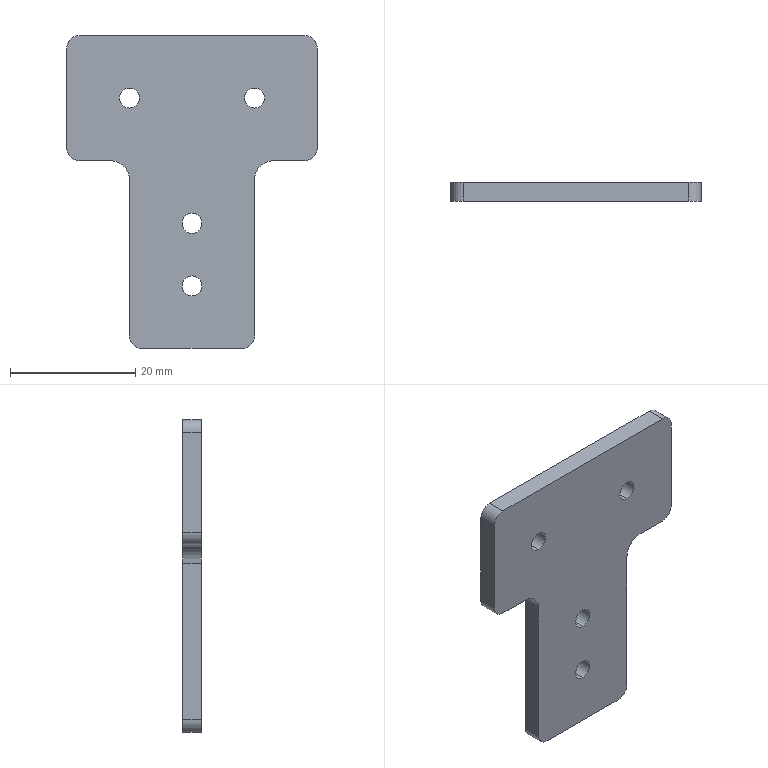Part | SolidWorks | features BaseBody 1 | 1 solid | 26 faces | box 40 x 3 x 50 mm | volume 4100 mm3 | cylinder 16 | plane 10 | commonest cylinder face diameters 3.2 x8 4 x6 6 x2
STEP:
#1=CARTESIAN_POINT('',(-10.,3.,16.6));
#2=VERTEX_POINT('',#1);
#3=CARTESIAN_POINT('',(-10.,3.,13.4));
#4=VERTEX_POINT('',#3);
#5=CARTESIAN_POINT('',(-10.,3.,15.));
#6=DIRECTION('',(0.,-1.,0.));
#7=DIRECTION('',(0.,0.,-1.));
#8=AXIS2_PLACEMENT_3D('',#5,#6,#7);
#9=CIRCLE('',#8,1.6);
#10=EDGE_CURVE('',#2,#4,#9,.T.);
#11=ORIENTED_EDGE('',*,*,#10,.F.);
#12=CARTESIAN_POINT('',(-10.,0.,16.6));
#13=VERTEX_POINT('',#12);
#14=CARTESIAN_POINT('',(-10.,3.,16.6));
#15=DIRECTION('',(0.,-1.,0.));
#16=VECTOR('',#15,1000.);
#17=LINE('',#14,#16);
#18=EDGE_CURVE('',#2,#13,#17,.T.);
#19=ORIENTED_EDGE('',*,*,#18,.T.);
#20=CARTESIAN_POINT('',(-10.,0.,13.4));
#21=VERTEX_POINT('',#20);
#22=CARTESIAN_POINT('',(-10.,0.,15.));
#23=DIRECTION('',(0.,-1.,0.));
#24=DIRECTION('',(0.,0.,-1.));
#25=AXIS2_PLACEMENT_3D('',#22,#23,#24);
#26=CIRCLE('',#25,1.6);
#27=EDGE_CURVE('',#13,#21,#26,.T.);
#28=ORIENTED_EDGE('',*,*,#27,.T.);
#29=CARTESIAN_POINT('',(-10.,3.,13.4));
#30=DIRECTION('',(0.,-1.,0.));
#31=VECTOR('',#30,1000.);
#32=LINE('',#29,#31);
#33=EDGE_CURVE('',#4,#21,#32,.T.);
#34=ORIENTED_EDGE('',*,*,#33,.F.);
#35=EDGE_LOOP('',(#11,#19,#28,#34));
#36=FACE_OUTER_BOUND('',#35,.T.);
#37=CARTESIAN_POINT('',(-10.,3.,15.));
#38=DIRECTION('',(0.,-1.,0.));
#39=DIRECTION('',(0.,0.,-1.));
#40=AXIS2_PLACEMENT_3D('',#37,#38,#39);
#41=CYLINDRICAL_SURFACE('',#40,1.6);
#42=ADVANCED_FACE('',(#36),#41,.F.);
#43=CARTESIAN_POINT('',(0.,3.,-13.4));
#44=VERTEX_POINT('',#43);
#45=CARTESIAN_POINT('',(0.,3.,-16.6));
#46=VERTEX_POINT('',#45);
#47=CARTESIAN_POINT('',(0.,3.,-15.));
#48=DIRECTION('',(0.,-1.,0.));
#49=DIRECTION('',(0.,0.,-1.));
#50=AXIS2_PLACEMENT_3D('',#47,#48,#49);
#51=CIRCLE('',#50,1.6);
#52=EDGE_CURVE('',#44,#46,#51,.T.);
#53=ORIENTED_EDGE('',*,*,#52,.F.);
#54=CARTESIAN_POINT('',(0.,0.,-13.4));
#55=VERTEX_POINT('',#54);
#56=CARTESIAN_POINT('',(0.,3.,-13.4));
#57=DIRECTION('',(0.,-1.,0.));
#58=VECTOR('',#57,1000.);
#59=LINE('',#56,#58);
#60=EDGE_CURVE('',#44,#55,#59,.T.);
#61=ORIENTED_EDGE('',*,*,#60,.T.);
#62=CARTESIAN_POINT('',(0.,0.,-16.6));
#63=VERTEX_POINT('',#62);
#64=CARTESIAN_POINT('',(0.,0.,-15.));
#65=DIRECTION('',(0.,-1.,0.));
#66=DIRECTION('',(0.,0.,-1.));
#67=AXIS2_PLACEMENT_3D('',#64,#65,#66);
#68=CIRCLE('',#67,1.6);
#69=EDGE_CURVE('',#55,#63,#68,.T.);
#70=ORIENTED_EDGE('',*,*,#69,.T.);
#71=CARTESIAN_POINT('',(0.,3.,-16.6));
#72=DIRECTION('',(0.,-1.,0.));
#73=VECTOR('',#72,1000.);
#74=LINE('',#71,#73);
#75=EDGE_CURVE('',#46,#63,#74,.T.);
#76=ORIENTED_EDGE('',*,*,#75,.F.);
#77=EDGE_LOOP('',(#53,#61,#70,#76));
#78=FACE_OUTER_BOUND('',#77,.T.);
#79=CARTESIAN_POINT('',(0.,3.,-15.));
#80=DIRECTION('',(0.,-1.,0.));
#81=DIRECTION('',(0.,0.,-1.));
#82=AXIS2_PLACEMENT_3D('',#79,#80,#81);
#83=CYLINDRICAL_SURFACE('',#82,1.6);
#84=ADVANCED_FACE('',(#78),#83,.F.);
#85=CARTESIAN_POINT('',(0.,3.,-3.4));
#86=VERTEX_POINT('',#85);
#87=CARTESIAN_POINT('',(0.,3.,-6.6));
#88=VERTEX_POINT('',#87);
#89=CARTESIAN_POINT('',(0.,3.,-5.));
#90=DIRECTION('',(0.,-1.,0.));
#91=DIRECTION('',(0.,0.,-1.));
#92=AXIS2_PLACEMENT_3D('',#89,#90,#91);
#93=CIRCLE('',#92,1.6);
#94=EDGE_CURVE('',#86,#88,#93,.T.);
#95=ORIENTED_EDGE('',*,*,#94,.F.);
#96=CARTESIAN_POINT('',(0.,0.,-3.4));
#97=VERTEX_POINT('',#96);
#98=CARTESIAN_POINT('',(0.,3.,-3.4));
#99=DIRECTION('',(0.,-1.,0.));
#100=VECTOR('',#99,1000.);
#101=LINE('',#98,#100);
#102=EDGE_CURVE('',#86,#97,#101,.T.);
#103=ORIENTED_EDGE('',*,*,#102,.T.);
#104=CARTESIAN_POINT('',(0.,0.,-6.6));
#105=VERTEX_POINT('',#104);
#106=CARTESIAN_POINT('',(0.,0.,-5.));
#107=DIRECTION('',(0.,-1.,0.));
#108=DIRECTION('',(0.,0.,-1.));
#109=AXIS2_PLACEMENT_3D('',#106,#107,#108);
#110=CIRCLE('',#109,1.6);
#111=EDGE_CURVE('',#97,#105,#110,.T.);
#112=ORIENTED_EDGE('',*,*,#111,.T.);
#113=CARTESIAN_POINT('',(0.,3.,-6.6));
#114=DIRECTION('',(0.,-1.,0.));
#115=VECTOR('',#114,1000.);
#116=LINE('',#113,#115);
#117=EDGE_CURVE('',#88,#105,#116,.T.);
#118=ORIENTED_EDGE('',*,*,#117,.F.);
#119=EDGE_LOOP('',(#95,#103,#112,#118));
#120=FACE_OUTER_BOUND('',#119,.T.);
#121=CARTESIAN_POINT('',(0.,3.,-5.));
#122=DIRECTION('',(0.,-1.,0.));
#123=DIRECTION('',(0.,0.,-1.));
#124=AXIS2_PLACEMENT_3D('',#121,#122,#123);
#125=CYLINDRICAL_SURFACE('',#124,1.6);
#126=ADVANCED_FACE('',(#120),#125,.F.);
#127=CARTESIAN_POINT('',(10.,3.,16.6));
#128=VERTEX_POINT('',#127);
#129=CARTESIAN_POINT('',(10.,3.,13.4));
#130=VERTEX_POINT('',#129);
#131=CARTESIAN_POINT('',(10.,3.,15.));
#132=DIRECTION('',(0.,-1.,0.));
#133=DIRECTION('',(0.,0.,-1.));
#134=AXIS2_PLACEMENT_3D('',#131,#132,#133);
#135=CIRCLE('',#134,1.6);
#136=EDGE_CURVE('',#128,#130,#135,.T.);
#137=ORIENTED_EDGE('',*,*,#136,.F.);
#138=CARTESIAN_POINT('',(10.,0.,16.6));
#139=VERTEX_POINT('',#138);
#140=CARTESIAN_POINT('',(10.,3.,16.6));
#141=DIRECTION('',(0.,-1.,0.));
#142=VECTOR('',#141,1000.);
#143=LINE('',#140,#142);
#144=EDGE_CURVE('',#128,#139,#143,.T.);
#145=ORIENTED_EDGE('',*,*,#144,.T.);
#146=CARTESIAN_POINT('',(10.,0.,13.4));
#147=VERTEX_POINT('',#146);
#148=CARTESIAN_POINT('',(10.,0.,15.));
#149=DIRECTION('',(0.,-1.,0.));
#150=DIRECTION('',(0.,0.,-1.));
#151=AXIS2_PLACEMENT_3D('',#148,#149,#150);
#152=CIRCLE('',#151,1.6);
#153=EDGE_CURVE('',#139,#147,#152,.T.);
#154=ORIENTED_EDGE('',*,*,#153,.T.);
#155=CARTESIAN_POINT('',(10.,3.,13.4));
#156=DIRECTION('',(0.,-1.,0.));
#157=VECTOR('',#156,1000.);
#158=LINE('',#155,#157);
#159=EDGE_CURVE('',#130,#147,#158,.T.);
#160=ORIENTED_EDGE('',*,*,#159,.F.);
#161=EDGE_LOOP('',(#137,#145,#154,#160));
#162=FACE_OUTER_BOUND('',#161,.T.);
#163=CARTESIAN_POINT('',(10.,3.,15.));
#164=DIRECTION('',(0.,-1.,0.));
#165=DIRECTION('',(0.,0.,-1.));
#166=AXIS2_PLACEMENT_3D('',#163,#164,#165);
#167=CYLINDRICAL_SURFACE('',#166,1.6);
#168=ADVANCED_FACE('',(#162),#167,.F.);
#169=CARTESIAN_POINT('',(-10.,0.,15.));
#170=DIRECTION('',(0.,-1.,0.));
#171=DIRECTION('',(0.,0.,-1.));
#172=AXIS2_PLACEMENT_3D('',#169,#170,#171);
#173=CIRCLE('',#172,1.6);
#174=EDGE_CURVE('',#21,#13,#173,.T.);
#175=ORIENTED_EDGE('',*,*,#174,.F.);
#176=ORIENTED_EDGE('',*,*,#27,.F.);
#177=EDGE_LOOP('',(#175,#176));
#178=FACE_BOUND('',#177,.T.);
#179=CARTESIAN_POINT('',(0.,0.,-15.));
#180=DIRECTION('',(0.,-1.,0.));
#181=DIRECTION('',(0.,0.,-1.));
#182=AXIS2_PLACEMENT_3D('',#179,#180,#181);
#183=CIRCLE('',#182,1.6);
#184=EDGE_CURVE('',#63,#55,#183,.T.);
#185=ORIENTED_EDGE('',*,*,#184,.F.);
#186=ORIENTED_EDGE('',*,*,#69,.F.);
#187=EDGE_LOOP('',(#185,#186));
#188=FACE_BOUND('',#187,.T.);
#189=CARTESIAN_POINT('',(0.,0.,-5.));
#190=DIRECTION('',(0.,-1.,0.));
#191=DIRECTION('',(0.,0.,-1.));
#192=AXIS2_PLACEMENT_3D('',#189,#190,#191);
#193=CIRCLE('',#192,1.6);
#194=EDGE_CURVE('',#105,#97,#193,.T.);
#195=ORIENTED_EDGE('',*,*,#194,.F.);
#196=ORIENTED_EDGE('',*,*,#111,.F.);
#197=EDGE_LOOP('',(#195,#196));
#198=FACE_BOUND('',#197,.T.);
#199=CARTESIAN_POINT('',(10.,0.,15.));
#200=DIRECTION('',(0.,-1.,0.));
#201=DIRECTION('',(0.,0.,-1.));
#202=AXIS2_PLACEMENT_3D('',#199,#200,#201);
#203=CIRCLE('',#202,1.6);
#204=EDGE_CURVE('',#147,#139,#203,.T.);
#205=ORIENTED_EDGE('',*,*,#204,.F.);
#206=ORIENTED_EDGE('',*,*,#153,.F.);
#207=EDGE_LOOP('',(#205,#206));
#208=FACE_BOUND('',#207,.T.);
#209=CARTESIAN_POINT('',(-18.,0.,5.));
#210=VERTEX_POINT('',#209);
#211=CARTESIAN_POINT('',(-20.,0.,7.));
#212=VERTEX_POINT('',#211);
#213=CARTESIAN_POINT('',(-18.,0.,7.));
#214=DIRECTION('',(0.,1.,0.));
#215=DIRECTION('',(0.,0.,1.));
#216=AXIS2_PLACEMENT_3D('',#213,#214,#215);
#217=CIRCLE('',#216,2.);
#218=EDGE_CURVE('',#210,#212,#217,.T.);
#219=ORIENTED_EDGE('',*,*,#218,.F.);
#220=CARTESIAN_POINT('',(-13.,0.,5.));
#221=VERTEX_POINT('',#220);
#222=CARTESIAN_POINT('',(0.,0.,5.));
#223=DIRECTION('',(-1.,0.,0.));
#224=VECTOR('',#223,1000.);
#225=LINE('',#222,#224);
#226=EDGE_CURVE('',#221,#210,#225,.T.);
#227=ORIENTED_EDGE('',*,*,#226,.F.);
#228=CARTESIAN_POINT('',(-10.,0.,2.));
#229=VERTEX_POINT('',#228);
#230=CARTESIAN_POINT('',(-13.,0.,2.));
#231=DIRECTION('',(0.,-1.,0.));
#232=DIRECTION('',(0.,0.,-1.));
#233=AXIS2_PLACEMENT_3D('',#230,#231,#232);
#234=CIRCLE('',#233,3.);
#235=EDGE_CURVE('',#229,#221,#234,.T.);
#236=ORIENTED_EDGE('',*,*,#235,.F.);
#237=CARTESIAN_POINT('',(-10.,0.,-23.));
#238=VERTEX_POINT('',#237);
#239=CARTESIAN_POINT('',(-10.,0.,0.));
#240=DIRECTION('',(0.,0.,1.));
#241=VECTOR('',#240,1000.);
#242=LINE('',#239,#241);
#243=EDGE_CURVE('',#238,#229,#242,.T.);
#244=ORIENTED_EDGE('',*,*,#243,.F.);
#245=CARTESIAN_POINT('',(-8.,0.,-25.));
#246=VERTEX_POINT('',#245);
#247=CARTESIAN_POINT('',(-8.,0.,-23.));
#248=DIRECTION('',(0.,1.,0.));
#249=DIRECTION('',(0.,0.,-1.));
#250=AXIS2_PLACEMENT_3D('',#247,#248,#249);
#251=CIRCLE('',#250,2.);
#252=EDGE_CURVE('',#246,#238,#251,.T.);
#253=ORIENTED_EDGE('',*,*,#252,.F.);
#254=CARTESIAN_POINT('',(8.,0.,-25.));
#255=VERTEX_POINT('',#254);
#256=CARTESIAN_POINT('',(0.,0.,-25.));
#257=DIRECTION('',(-1.,0.,0.));
#258=VECTOR('',#257,1000.);
#259=LINE('',#256,#258);
#260=EDGE_CURVE('',#255,#246,#259,.T.);
#261=ORIENTED_EDGE('',*,*,#260,.F.);
#262=CARTESIAN_POINT('',(10.,0.,-23.));
#263=VERTEX_POINT('',#262);
#264=CARTESIAN_POINT('',(8.,0.,-23.));
#265=DIRECTION('',(0.,1.,0.));
#266=DIRECTION('',(0.,0.,1.));
#267=AXIS2_PLACEMENT_3D('',#264,#265,#266);
#268=CIRCLE('',#267,2.);
#269=EDGE_CURVE('',#263,#255,#268,.T.);
#270=ORIENTED_EDGE('',*,*,#269,.F.);
#271=CARTESIAN_POINT('',(10.,0.,2.));
#272=VERTEX_POINT('',#271);
#273=CARTESIAN_POINT('',(10.,0.,0.));
#274=DIRECTION('',(0.,0.,-1.));
#275=VECTOR('',#274,1000.);
#276=LINE('',#273,#275);
#277=EDGE_CURVE('',#272,#263,#276,.T.);
#278=ORIENTED_EDGE('',*,*,#277,.F.);
#279=CARTESIAN_POINT('',(13.,0.,5.));
#280=VERTEX_POINT('',#279);
#281=CARTESIAN_POINT('',(13.,0.,2.));
#282=DIRECTION('',(0.,-1.,0.));
#283=DIRECTION('',(0.,0.,1.));
#284=AXIS2_PLACEMENT_3D('',#281,#282,#283);
#285=CIRCLE('',#284,3.);
#286=EDGE_CURVE('',#280,#272,#285,.T.);
#287=ORIENTED_EDGE('',*,*,#286,.F.);
#288=CARTESIAN_POINT('',(18.,0.,5.));
#289=VERTEX_POINT('',#288);
#290=CARTESIAN_POINT('',(0.,0.,5.));
#291=DIRECTION('',(-1.,0.,0.));
#292=VECTOR('',#291,1000.);
#293=LINE('',#290,#292);
#294=EDGE_CURVE('',#289,#280,#293,.T.);
#295=ORIENTED_EDGE('',*,*,#294,.F.);
#296=CARTESIAN_POINT('',(20.,0.,7.));
#297=VERTEX_POINT('',#296);
#298=CARTESIAN_POINT('',(18.,0.,7.));
#299=DIRECTION('',(0.,1.,0.));
#300=DIRECTION('',(0.,0.,-1.));
#301=AXIS2_PLACEMENT_3D('',#298,#299,#300);
#302=CIRCLE('',#301,2.);
#303=EDGE_CURVE('',#297,#289,#302,.T.);
#304=ORIENTED_EDGE('',*,*,#303,.F.);
#305=CARTESIAN_POINT('',(20.,0.,23.));
#306=VERTEX_POINT('',#305);
#307=CARTESIAN_POINT('',(20.,0.,0.));
#308=DIRECTION('',(0.,0.,-1.));
#309=VECTOR('',#308,1000.);
#310=LINE('',#307,#309);
#311=EDGE_CURVE('',#306,#297,#310,.T.);
#312=ORIENTED_EDGE('',*,*,#311,.F.);
#313=CARTESIAN_POINT('',(18.,0.,25.));
#314=VERTEX_POINT('',#313);
#315=CARTESIAN_POINT('',(18.,0.,23.));
#316=DIRECTION('',(0.,1.,0.));
#317=DIRECTION('',(0.,0.,-1.));
#318=AXIS2_PLACEMENT_3D('',#315,#316,#317);
#319=CIRCLE('',#318,2.);
#320=EDGE_CURVE('',#314,#306,#319,.T.);
#321=ORIENTED_EDGE('',*,*,#320,.F.);
#322=CARTESIAN_POINT('',(-18.,0.,25.));
#323=VERTEX_POINT('',#322);
#324=CARTESIAN_POINT('',(0.,0.,25.));
#325=DIRECTION('',(1.,0.,0.));
#326=VECTOR('',#325,1000.);
#327=LINE('',#324,#326);
#328=EDGE_CURVE('',#323,#314,#327,.T.);
#329=ORIENTED_EDGE('',*,*,#328,.F.);
#330=CARTESIAN_POINT('',(-20.,0.,23.));
#331=VERTEX_POINT('',#330);
#332=CARTESIAN_POINT('',(-18.,0.,23.));
#333=DIRECTION('',(0.,1.,0.));
#334=DIRECTION('',(0.,0.,1.));
#335=AXIS2_PLACEMENT_3D('',#332,#333,#334);
#336=CIRCLE('',#335,2.);
#337=EDGE_CURVE('',#331,#323,#336,.T.);
#338=ORIENTED_EDGE('',*,*,#337,.F.);
#339=CARTESIAN_POINT('',(-20.,0.,0.));
#340=DIRECTION('',(0.,0.,1.));
#341=VECTOR('',#340,1000.);
#342=LINE('',#339,#341);
#343=EDGE_CURVE('',#212,#331,#342,.T.);
#344=ORIENTED_EDGE('',*,*,#343,.F.);
#345=EDGE_LOOP('',(#219,#227,#236,#244,#253,#261,#270,#278,#287,#295,#304,#312,#321,#329,#338,#344));
#346=FACE_OUTER_BOUND('',#345,.T.);
#347=CARTESIAN_POINT('',(0.,0.,0.));
#348=DIRECTION('',(0.,1.,0.));
#349=DIRECTION('',(0.,0.,1.));
#350=AXIS2_PLACEMENT_3D('',#347,#348,#349);
#351=PLANE('',#350);
#352=ADVANCED_FACE('',(#178,#188,#198,#208,#346),#351,.F.);
#353=ORIENTED_EDGE('',*,*,#18,.F.);
#354=CARTESIAN_POINT('',(-10.,3.,15.));
#355=DIRECTION('',(0.,-1.,0.));
#356=DIRECTION('',(0.,0.,-1.));
#357=AXIS2_PLACEMENT_3D('',#354,#355,#356);
#358=CIRCLE('',#357,1.6);
#359=EDGE_CURVE('',#4,#2,#358,.T.);
#360=ORIENTED_EDGE('',*,*,#359,.F.);
#361=ORIENTED_EDGE('',*,*,#33,.T.);
#362=ORIENTED_EDGE('',*,*,#174,.T.);
#363=EDGE_LOOP('',(#353,#360,#361,#362));
#364=FACE_OUTER_BOUND('',#363,.T.);
#365=CARTESIAN_POINT('',(-10.,3.,15.));
#366=DIRECTION('',(0.,-1.,0.));
#367=DIRECTION('',(0.,0.,-1.));
#368=AXIS2_PLACEMENT_3D('',#365,#366,#367);
#369=CYLINDRICAL_SURFACE('',#368,1.6);
#370=ADVANCED_FACE('',(#364),#369,.F.);
#371=ORIENTED_EDGE('',*,*,#60,.F.);
#372=CARTESIAN_POINT('',(0.,3.,-15.));
#373=DIRECTION('',(0.,-1.,0.));
#374=DIRECTION('',(0.,0.,-1.));
#375=AXIS2_PLACEMENT_3D('',#372,#373,#374);
#376=CIRCLE('',#375,1.6);
#377=EDGE_CURVE('',#46,#44,#376,.T.);
#378=ORIENTED_EDGE('',*,*,#377,.F.);
#379=ORIENTED_EDGE('',*,*,#75,.T.);
#380=ORIENTED_EDGE('',*,*,#184,.T.);
#381=EDGE_LOOP('',(#371,#378,#379,#380));
#382=FACE_OUTER_BOUND('',#381,.T.);
#383=CARTESIAN_POINT('',(0.,3.,-15.));
#384=DIRECTION('',(0.,-1.,0.));
#385=DIRECTION('',(0.,0.,-1.));
#386=AXIS2_PLACEMENT_3D('',#383,#384,#385);
#387=CYLINDRICAL_SURFACE('',#386,1.6);
#388=ADVANCED_FACE('',(#382),#387,.F.);
#389=ORIENTED_EDGE('',*,*,#102,.F.);
#390=CARTESIAN_POINT('',(0.,3.,-5.));
#391=DIRECTION('',(0.,-1.,0.));
#392=DIRECTION('',(0.,0.,-1.));
#393=AXIS2_PLACEMENT_3D('',#390,#391,#392);
#394=CIRCLE('',#393,1.6);
#395=EDGE_CURVE('',#88,#86,#394,.T.);
#396=ORIENTED_EDGE('',*,*,#395,.F.);
#397=ORIENTED_EDGE('',*,*,#117,.T.);
#398=ORIENTED_EDGE('',*,*,#194,.T.);
#399=EDGE_LOOP('',(#389,#396,#397,#398));
#400=FACE_OUTER_BOUND('',#399,.T.);
#401=CARTESIAN_POINT('',(0.,3.,-5.));
#402=DIRECTION('',(0.,-1.,0.));
#403=DIRECTION('',(0.,0.,-1.));
#404=AXIS2_PLACEMENT_3D('',#401,#402,#403);
#405=CYLINDRICAL_SURFACE('',#404,1.6);
#406=ADVANCED_FACE('',(#400),#405,.F.);
#407=ORIENTED_EDGE('',*,*,#144,.F.);
#408=CARTESIAN_POINT('',(10.,3.,15.));
#409=DIRECTION('',(0.,-1.,0.));
#410=DIRECTION('',(0.,0.,-1.));
#411=AXIS2_PLACEMENT_3D('',#408,#409,#410);
#412=CIRCLE('',#411,1.6);
#413=EDGE_CURVE('',#130,#128,#412,.T.);
#414=ORIENTED_EDGE('',*,*,#413,.F.);
#415=ORIENTED_EDGE('',*,*,#159,.T.);
#416=ORIENTED_EDGE('',*,*,#204,.T.);
#417=EDGE_LOOP('',(#407,#414,#415,#416));
#418=FACE_OUTER_BOUND('',#417,.T.);
#419=CARTESIAN_POINT('',(10.,3.,15.));
#420=DIRECTION('',(0.,-1.,0.));
#421=DIRECTION('',(0.,0.,-1.));
#422=AXIS2_PLACEMENT_3D('',#419,#420,#421);
#423=CYLINDRICAL_SURFACE('',#422,1.6);
#424=ADVANCED_FACE('',(#418),#423,.F.);
#425=ORIENTED_EDGE('',*,*,#343,.T.);
#426=CARTESIAN_POINT('',(-20.,3.,23.));
#427=VERTEX_POINT('',#426);
#428=CARTESIAN_POINT('',(-20.,3.,23.));
#429=DIRECTION('',(0.,1.,0.));
#430=VECTOR('',#429,1000.);
#431=LINE('',#428,#430);
#432=EDGE_CURVE('',#331,#427,#431,.T.);
#433=ORIENTED_EDGE('',*,*,#432,.T.);
#434=CARTESIAN_POINT('',(-20.,3.,7.));
#435=VERTEX_POINT('',#434);
#436=CARTESIAN_POINT('',(-20.,3.,0.));
#437=DIRECTION('',(0.,0.,-1.));
#438=VECTOR('',#437,1000.);
#439=LINE('',#436,#438);
#440=EDGE_CURVE('',#427,#435,#439,.T.);
#441=ORIENTED_EDGE('',*,*,#440,.T.);
#442=CARTESIAN_POINT('',(-20.,3.,7.));
#443=DIRECTION('',(0.,-1.,0.));
#444=VECTOR('',#443,1000.);
#445=LINE('',#442,#444);
#446=EDGE_CURVE('',#435,#212,#445,.T.);
#447=ORIENTED_EDGE('',*,*,#446,.T.);
#448=EDGE_LOOP('',(#425,#433,#441,#447));
#449=FACE_OUTER_BOUND('',#448,.T.);
#450=CARTESIAN_POINT('',(-20.,3.,0.));
#451=DIRECTION('',(-1.,0.,0.));
#452=DIRECTION('',(0.,0.,1.));
#453=AXIS2_PLACEMENT_3D('',#450,#451,#452);
#454=PLANE('',#453);
#455=ADVANCED_FACE('',(#449),#454,.T.);
#456=ORIENTED_EDGE('',*,*,#218,.T.);
#457=ORIENTED_EDGE('',*,*,#446,.F.);
#458=CARTESIAN_POINT('',(-18.,3.,5.));
#459=VERTEX_POINT('',#458);
#460=CARTESIAN_POINT('',(-18.,3.,7.));
#461=DIRECTION('',(0.,-1.,0.));
#462=DIRECTION('',(0.,0.,1.));
#463=AXIS2_PLACEMENT_3D('',#460,#461,#462);
#464=CIRCLE('',#463,2.);
#465=EDGE_CURVE('',#435,#459,#464,.T.);
#466=ORIENTED_EDGE('',*,*,#465,.T.);
#467=CARTESIAN_POINT('',(-18.,3.,5.));
#468=DIRECTION('',(0.,-1.,0.));
#469=VECTOR('',#468,1000.);
#470=LINE('',#467,#469);
#471=EDGE_CURVE('',#459,#210,#470,.T.);
#472=ORIENTED_EDGE('',*,*,#471,.T.);
#473=EDGE_LOOP('',(#456,#457,#466,#472));
#474=FACE_OUTER_BOUND('',#473,.T.);
#475=CARTESIAN_POINT('',(-18.,3.,7.));
#476=DIRECTION('',(0.,1.,0.));
#477=DIRECTION('',(0.,0.,1.));
#478=AXIS2_PLACEMENT_3D('',#475,#476,#477);
#479=CYLINDRICAL_SURFACE('',#478,2.);
#480=ADVANCED_FACE('',(#474),#479,.T.);
#481=ORIENTED_EDGE('',*,*,#471,.F.);
#482=CARTESIAN_POINT('',(-13.,3.,5.));
#483=VERTEX_POINT('',#482);
#484=CARTESIAN_POINT('',(0.,3.,5.));
#485=DIRECTION('',(-1.,0.,0.));
#486=VECTOR('',#485,1000.);
#487=LINE('',#484,#486);
#488=EDGE_CURVE('',#483,#459,#487,.T.);
#489=ORIENTED_EDGE('',*,*,#488,.F.);
#490=CARTESIAN_POINT('',(-13.,3.,5.));
#491=DIRECTION('',(0.,1.,0.));
#492=VECTOR('',#491,1000.);
#493=LINE('',#490,#492);
#494=EDGE_CURVE('',#221,#483,#493,.T.);
#495=ORIENTED_EDGE('',*,*,#494,.F.);
#496=ORIENTED_EDGE('',*,*,#226,.T.);
#497=EDGE_LOOP('',(#481,#489,#495,#496));
#498=FACE_OUTER_BOUND('',#497,.T.);
#499=CARTESIAN_POINT('',(0.,3.,5.));
#500=DIRECTION('',(0.,0.,1.));
#501=DIRECTION('',(1.,0.,0.));
#502=AXIS2_PLACEMENT_3D('',#499,#500,#501);
#503=PLANE('',#502);
#504=ADVANCED_FACE('',(#498),#503,.F.);
#505=CARTESIAN_POINT('',(-10.,3.,2.));
#506=VERTEX_POINT('',#505);
#507=CARTESIAN_POINT('',(-10.,3.,2.));
#508=DIRECTION('',(0.,1.,0.));
#509=VECTOR('',#508,1000.);
#510=LINE('',#507,#509);
#511=EDGE_CURVE('',#229,#506,#510,.T.);
#512=ORIENTED_EDGE('',*,*,#511,.F.);
#513=ORIENTED_EDGE('',*,*,#235,.T.);
#514=ORIENTED_EDGE('',*,*,#494,.T.);
#515=CARTESIAN_POINT('',(-13.,3.,2.));
#516=DIRECTION('',(0.,-1.,0.));
#517=DIRECTION('',(0.,0.,-1.));
#518=AXIS2_PLACEMENT_3D('',#515,#516,#517);
#519=CIRCLE('',#518,3.);
#520=EDGE_CURVE('',#506,#483,#519,.T.);
#521=ORIENTED_EDGE('',*,*,#520,.F.);
#522=EDGE_LOOP('',(#512,#513,#514,#521));
#523=FACE_OUTER_BOUND('',#522,.T.);
#524=CARTESIAN_POINT('',(-13.,3.,2.));
#525=DIRECTION('',(0.,-1.,0.));
#526=DIRECTION('',(0.,0.,-1.));
#527=AXIS2_PLACEMENT_3D('',#524,#525,#526);
#528=CYLINDRICAL_SURFACE('',#527,3.);
#529=ADVANCED_FACE('',(#523),#528,.F.);
#530=ORIENTED_EDGE('',*,*,#243,.T.);
#531=ORIENTED_EDGE('',*,*,#511,.T.);
#532=CARTESIAN_POINT('',(-10.,3.,-23.));
#533=VERTEX_POINT('',#532);
#534=CARTESIAN_POINT('',(-10.,3.,0.));
#535=DIRECTION('',(0.,0.,-1.));
#536=VECTOR('',#535,1000.);
#537=LINE('',#534,#536);
#538=EDGE_CURVE('',#506,#533,#537,.T.);
#539=ORIENTED_EDGE('',*,*,#538,.T.);
#540=CARTESIAN_POINT('',(-10.,3.,-23.));
#541=DIRECTION('',(0.,-1.,0.));
#542=VECTOR('',#541,1000.);
#543=LINE('',#540,#542);
#544=EDGE_CURVE('',#533,#238,#543,.T.);
#545=ORIENTED_EDGE('',*,*,#544,.T.);
#546=EDGE_LOOP('',(#530,#531,#539,#545));
#547=FACE_OUTER_BOUND('',#546,.T.);
#548=CARTESIAN_POINT('',(-10.,3.,0.));
#549=DIRECTION('',(-1.,0.,0.));
#550=DIRECTION('',(0.,0.,1.));
#551=AXIS2_PLACEMENT_3D('',#548,#549,#550);
#552=PLANE('',#551);
#553=ADVANCED_FACE('',(#547),#552,.T.);
#554=ORIENTED_EDGE('',*,*,#252,.T.);
#555=ORIENTED_EDGE('',*,*,#544,.F.);
#556=CARTESIAN_POINT('',(-8.,3.,-25.));
#557=VERTEX_POINT('',#556);
#558=CARTESIAN_POINT('',(-8.,3.,-23.));
#559=DIRECTION('',(0.,-1.,0.));
#560=DIRECTION('',(0.,0.,-1.));
#561=AXIS2_PLACEMENT_3D('',#558,#559,#560);
#562=CIRCLE('',#561,2.);
#563=EDGE_CURVE('',#533,#557,#562,.T.);
#564=ORIENTED_EDGE('',*,*,#563,.T.);
#565=CARTESIAN_POINT('',(-8.,3.,-25.));
#566=DIRECTION('',(0.,-1.,0.));
#567=VECTOR('',#566,1000.);
#568=LINE('',#565,#567);
#569=EDGE_CURVE('',#557,#246,#568,.T.);
#570=ORIENTED_EDGE('',*,*,#569,.T.);
#571=EDGE_LOOP('',(#554,#555,#564,#570));
#572=FACE_OUTER_BOUND('',#571,.T.);
#573=CARTESIAN_POINT('',(-8.,3.,-23.));
#574=DIRECTION('',(0.,-1.,0.));
#575=DIRECTION('',(0.,0.,-1.));
#576=AXIS2_PLACEMENT_3D('',#573,#574,#575);
#577=CYLINDRICAL_SURFACE('',#576,2.);
#578=ADVANCED_FACE('',(#572),#577,.T.);
#579=ORIENTED_EDGE('',*,*,#260,.T.);
#580=ORIENTED_EDGE('',*,*,#569,.F.);
#581=CARTESIAN_POINT('',(8.,3.,-25.));
#582=VERTEX_POINT('',#581);
#583=CARTESIAN_POINT('',(0.,3.,-25.));
#584=DIRECTION('',(1.,0.,0.));
#585=VECTOR('',#584,1000.);
#586=LINE('',#583,#585);
#587=EDGE_CURVE('',#557,#582,#586,.T.);
#588=ORIENTED_EDGE('',*,*,#587,.T.);
#589=CARTESIAN_POINT('',(8.,3.,-25.));
#590=DIRECTION('',(0.,-1.,0.));
#591=VECTOR('',#590,1000.);
#592=LINE('',#589,#591);
#593=EDGE_CURVE('',#582,#255,#592,.T.);
#594=ORIENTED_EDGE('',*,*,#593,.T.);
#595=EDGE_LOOP('',(#579,#580,#588,#594));
#596=FACE_OUTER_BOUND('',#595,.T.);
#597=CARTESIAN_POINT('',(0.,3.,-25.));
#598=DIRECTION('',(0.,0.,-1.));
#599=DIRECTION('',(-1.,0.,0.));
#600=AXIS2_PLACEMENT_3D('',#597,#598,#599);
#601=PLANE('',#600);
#602=ADVANCED_FACE('',(#596),#601,.T.);
#603=ORIENTED_EDGE('',*,*,#269,.T.);
#604=ORIENTED_EDGE('',*,*,#593,.F.);
#605=CARTESIAN_POINT('',(10.,3.,-23.));
#606=VERTEX_POINT('',#605);
#607=CARTESIAN_POINT('',(8.,3.,-23.));
#608=DIRECTION('',(0.,-1.,0.));
#609=DIRECTION('',(0.,0.,1.));
#610=AXIS2_PLACEMENT_3D('',#607,#608,#609);
#611=CIRCLE('',#610,2.);
#612=EDGE_CURVE('',#582,#606,#611,.T.);
#613=ORIENTED_EDGE('',*,*,#612,.T.);
#614=CARTESIAN_POINT('',(10.,3.,-23.));
#615=DIRECTION('',(0.,-1.,0.));
#616=VECTOR('',#615,1000.);
#617=LINE('',#614,#616);
#618=EDGE_CURVE('',#606,#263,#617,.T.);
#619=ORIENTED_EDGE('',*,*,#618,.T.);
#620=EDGE_LOOP('',(#603,#604,#613,#619));
#621=FACE_OUTER_BOUND('',#620,.T.);
#622=CARTESIAN_POINT('',(8.,3.,-23.));
#623=DIRECTION('',(0.,1.,0.));
#624=DIRECTION('',(0.,0.,1.));
#625=AXIS2_PLACEMENT_3D('',#622,#623,#624);
#626=CYLINDRICAL_SURFACE('',#625,2.);
#627=ADVANCED_FACE('',(#621),#626,.T.);
#628=ORIENTED_EDGE('',*,*,#618,.F.);
#629=CARTESIAN_POINT('',(10.,3.,2.));
#630=VERTEX_POINT('',#629);
#631=CARTESIAN_POINT('',(10.,3.,0.));
#632=DIRECTION('',(0.,0.,-1.));
#633=VECTOR('',#632,1000.);
#634=LINE('',#631,#633);
#635=EDGE_CURVE('',#630,#606,#634,.T.);
#636=ORIENTED_EDGE('',*,*,#635,.F.);
#637=CARTESIAN_POINT('',(10.,3.,2.));
#638=DIRECTION('',(0.,1.,0.));
#639=VECTOR('',#638,1000.);
#640=LINE('',#637,#639);
#641=EDGE_CURVE('',#272,#630,#640,.T.);
#642=ORIENTED_EDGE('',*,*,#641,.F.);
#643=ORIENTED_EDGE('',*,*,#277,.T.);
#644=EDGE_LOOP('',(#628,#636,#642,#643));
#645=FACE_OUTER_BOUND('',#644,.T.);
#646=CARTESIAN_POINT('',(10.,3.,0.));
#647=DIRECTION('',(-1.,0.,0.));
#648=DIRECTION('',(0.,0.,1.));
#649=AXIS2_PLACEMENT_3D('',#646,#647,#648);
#650=PLANE('',#649);
#651=ADVANCED_FACE('',(#645),#650,.F.);
#652=CARTESIAN_POINT('',(13.,3.,5.));
#653=VERTEX_POINT('',#652);
#654=CARTESIAN_POINT('',(13.,3.,5.));
#655=DIRECTION('',(0.,1.,0.));
#656=VECTOR('',#655,1000.);
#657=LINE('',#654,#656);
#658=EDGE_CURVE('',#280,#653,#657,.T.);
#659=ORIENTED_EDGE('',*,*,#658,.F.);
#660=ORIENTED_EDGE('',*,*,#286,.T.);
#661=ORIENTED_EDGE('',*,*,#641,.T.);
#662=CARTESIAN_POINT('',(13.,3.,2.));
#663=DIRECTION('',(0.,-1.,0.));
#664=DIRECTION('',(0.,0.,1.));
#665=AXIS2_PLACEMENT_3D('',#662,#663,#664);
#666=CIRCLE('',#665,3.);
#667=EDGE_CURVE('',#653,#630,#666,.T.);
#668=ORIENTED_EDGE('',*,*,#667,.F.);
#669=EDGE_LOOP('',(#659,#660,#661,#668));
#670=FACE_OUTER_BOUND('',#669,.T.);
#671=CARTESIAN_POINT('',(13.,3.,2.));
#672=DIRECTION('',(0.,1.,0.));
#673=DIRECTION('',(0.,0.,1.));
#674=AXIS2_PLACEMENT_3D('',#671,#672,#673);
#675=CYLINDRICAL_SURFACE('',#674,3.);
#676=ADVANCED_FACE('',(#670),#675,.F.);
#677=CARTESIAN_POINT('',(18.,3.,5.));
#678=VERTEX_POINT('',#677);
#679=CARTESIAN_POINT('',(18.,3.,5.));
#680=DIRECTION('',(0.,1.,0.));
#681=VECTOR('',#680,1000.);
#682=LINE('',#679,#681);
#683=EDGE_CURVE('',#289,#678,#682,.T.);
#684=ORIENTED_EDGE('',*,*,#683,.F.);
#685=ORIENTED_EDGE('',*,*,#294,.T.);
#686=ORIENTED_EDGE('',*,*,#658,.T.);
#687=CARTESIAN_POINT('',(0.,3.,5.));
#688=DIRECTION('',(-1.,0.,0.));
#689=VECTOR('',#688,1000.);
#690=LINE('',#687,#689);
#691=EDGE_CURVE('',#678,#653,#690,.T.);
#692=ORIENTED_EDGE('',*,*,#691,.F.);
#693=EDGE_LOOP('',(#684,#685,#686,#692));
#694=FACE_OUTER_BOUND('',#693,.T.);
#695=CARTESIAN_POINT('',(0.,3.,5.));
#696=DIRECTION('',(0.,0.,1.));
#697=DIRECTION('',(1.,0.,0.));
#698=AXIS2_PLACEMENT_3D('',#695,#696,#697);
#699=PLANE('',#698);
#700=ADVANCED_FACE('',(#694),#699,.F.);
#701=ORIENTED_EDGE('',*,*,#303,.T.);
#702=ORIENTED_EDGE('',*,*,#683,.T.);
#703=CARTESIAN_POINT('',(20.,3.,7.));
#704=VERTEX_POINT('',#703);
#705=CARTESIAN_POINT('',(18.,3.,7.));
#706=DIRECTION('',(0.,-1.,0.));
#707=DIRECTION('',(0.,0.,-1.));
#708=AXIS2_PLACEMENT_3D('',#705,#706,#707);
#709=CIRCLE('',#708,2.);
#710=EDGE_CURVE('',#678,#704,#709,.T.);
#711=ORIENTED_EDGE('',*,*,#710,.T.);
#712=CARTESIAN_POINT('',(20.,3.,7.));
#713=DIRECTION('',(0.,-1.,0.));
#714=VECTOR('',#713,1000.);
#715=LINE('',#712,#714);
#716=EDGE_CURVE('',#704,#297,#715,.T.);
#717=ORIENTED_EDGE('',*,*,#716,.T.);
#718=EDGE_LOOP('',(#701,#702,#711,#717));
#719=FACE_OUTER_BOUND('',#718,.T.);
#720=CARTESIAN_POINT('',(18.,3.,7.));
#721=DIRECTION('',(0.,-1.,0.));
#722=DIRECTION('',(0.,0.,-1.));
#723=AXIS2_PLACEMENT_3D('',#720,#721,#722);
#724=CYLINDRICAL_SURFACE('',#723,2.);
#725=ADVANCED_FACE('',(#719),#724,.T.);
#726=CARTESIAN_POINT('',(20.,3.,23.));
#727=VERTEX_POINT('',#726);
#728=CARTESIAN_POINT('',(20.,3.,23.));
#729=DIRECTION('',(0.,1.,0.));
#730=VECTOR('',#729,1000.);
#731=LINE('',#728,#730);
#732=EDGE_CURVE('',#306,#727,#731,.T.);
#733=ORIENTED_EDGE('',*,*,#732,.F.);
#734=ORIENTED_EDGE('',*,*,#311,.T.);
#735=ORIENTED_EDGE('',*,*,#716,.F.);
#736=CARTESIAN_POINT('',(20.,3.,0.));
#737=DIRECTION('',(0.,0.,-1.));
#738=VECTOR('',#737,1000.);
#739=LINE('',#736,#738);
#740=EDGE_CURVE('',#727,#704,#739,.T.);
#741=ORIENTED_EDGE('',*,*,#740,.F.);
#742=EDGE_LOOP('',(#733,#734,#735,#741));
#743=FACE_OUTER_BOUND('',#742,.T.);
#744=CARTESIAN_POINT('',(20.,3.,0.));
#745=DIRECTION('',(-1.,0.,0.));
#746=DIRECTION('',(0.,0.,1.));
#747=AXIS2_PLACEMENT_3D('',#744,#745,#746);
#748=PLANE('',#747);
#749=ADVANCED_FACE('',(#743),#748,.F.);
#750=ORIENTED_EDGE('',*,*,#320,.T.);
#751=ORIENTED_EDGE('',*,*,#732,.T.);
#752=CARTESIAN_POINT('',(18.,3.,25.));
#753=VERTEX_POINT('',#752);
#754=CARTESIAN_POINT('',(18.,3.,23.));
#755=DIRECTION('',(0.,-1.,0.));
#756=DIRECTION('',(0.,0.,-1.));
#757=AXIS2_PLACEMENT_3D('',#754,#755,#756);
#758=CIRCLE('',#757,2.);
#759=EDGE_CURVE('',#727,#753,#758,.T.);
#760=ORIENTED_EDGE('',*,*,#759,.T.);
#761=CARTESIAN_POINT('',(18.,3.,25.));
#762=DIRECTION('',(0.,-1.,0.));
#763=VECTOR('',#762,1000.);
#764=LINE('',#761,#763);
#765=EDGE_CURVE('',#753,#314,#764,.T.);
#766=ORIENTED_EDGE('',*,*,#765,.T.);
#767=EDGE_LOOP('',(#750,#751,#760,#766));
#768=FACE_OUTER_BOUND('',#767,.T.);
#769=CARTESIAN_POINT('',(18.,3.,23.));
#770=DIRECTION('',(0.,-1.,0.));
#771=DIRECTION('',(0.,0.,-1.));
#772=AXIS2_PLACEMENT_3D('',#769,#770,#771);
#773=CYLINDRICAL_SURFACE('',#772,2.);
#774=ADVANCED_FACE('',(#768),#773,.T.);
#775=CARTESIAN_POINT('',(-18.,3.,25.));
#776=VERTEX_POINT('',#775);
#777=CARTESIAN_POINT('',(-18.,3.,25.));
#778=DIRECTION('',(0.,1.,0.));
#779=VECTOR('',#778,1000.);
#780=LINE('',#777,#779);
#781=EDGE_CURVE('',#323,#776,#780,.T.);
#782=ORIENTED_EDGE('',*,*,#781,.F.);
#783=ORIENTED_EDGE('',*,*,#328,.T.);
#784=ORIENTED_EDGE('',*,*,#765,.F.);
#785=CARTESIAN_POINT('',(0.,3.,25.));
#786=DIRECTION('',(1.,0.,0.));
#787=VECTOR('',#786,1000.);
#788=LINE('',#785,#787);
#789=EDGE_CURVE('',#776,#753,#788,.T.);
#790=ORIENTED_EDGE('',*,*,#789,.F.);
#791=EDGE_LOOP('',(#782,#783,#784,#790));
#792=FACE_OUTER_BOUND('',#791,.T.);
#793=CARTESIAN_POINT('',(0.,3.,25.));
#794=DIRECTION('',(0.,0.,-1.));
#795=DIRECTION('',(-1.,0.,0.));
#796=AXIS2_PLACEMENT_3D('',#793,#794,#795);
#797=PLANE('',#796);
#798=ADVANCED_FACE('',(#792),#797,.F.);
#799=ORIENTED_EDGE('',*,*,#337,.T.);
#800=ORIENTED_EDGE('',*,*,#781,.T.);
#801=CARTESIAN_POINT('',(-18.,3.,23.));
#802=DIRECTION('',(0.,-1.,0.));
#803=DIRECTION('',(0.,0.,1.));
#804=AXIS2_PLACEMENT_3D('',#801,#802,#803);
#805=CIRCLE('',#804,2.);
#806=EDGE_CURVE('',#776,#427,#805,.T.);
#807=ORIENTED_EDGE('',*,*,#806,.T.);
#808=ORIENTED_EDGE('',*,*,#432,.F.);
#809=EDGE_LOOP('',(#799,#800,#807,#808));
#810=FACE_OUTER_BOUND('',#809,.T.);
#811=CARTESIAN_POINT('',(-18.,3.,23.));
#812=DIRECTION('',(0.,1.,0.));
#813=DIRECTION('',(0.,0.,1.));
#814=AXIS2_PLACEMENT_3D('',#811,#812,#813);
#815=CYLINDRICAL_SURFACE('',#814,2.);
#816=ADVANCED_FACE('',(#810),#815,.T.);
#817=ORIENTED_EDGE('',*,*,#359,.T.);
#818=ORIENTED_EDGE('',*,*,#10,.T.);
#819=EDGE_LOOP('',(#817,#818));
#820=FACE_BOUND('',#819,.T.);
#821=ORIENTED_EDGE('',*,*,#377,.T.);
#822=ORIENTED_EDGE('',*,*,#52,.T.);
#823=EDGE_LOOP('',(#821,#822));
#824=FACE_BOUND('',#823,.T.);
#825=ORIENTED_EDGE('',*,*,#395,.T.);
#826=ORIENTED_EDGE('',*,*,#94,.T.);
#827=EDGE_LOOP('',(#825,#826));
#828=FACE_BOUND('',#827,.T.);
#829=ORIENTED_EDGE('',*,*,#413,.T.);
#830=ORIENTED_EDGE('',*,*,#136,.T.);
#831=EDGE_LOOP('',(#829,#830));
#832=FACE_BOUND('',#831,.T.);
#833=ORIENTED_EDGE('',*,*,#538,.F.);
#834=ORIENTED_EDGE('',*,*,#520,.T.);
#835=ORIENTED_EDGE('',*,*,#488,.T.);
#836=ORIENTED_EDGE('',*,*,#465,.F.);
#837=ORIENTED_EDGE('',*,*,#440,.F.);
#838=ORIENTED_EDGE('',*,*,#806,.F.);
#839=ORIENTED_EDGE('',*,*,#789,.T.);
#840=ORIENTED_EDGE('',*,*,#759,.F.);
#841=ORIENTED_EDGE('',*,*,#740,.T.);
#842=ORIENTED_EDGE('',*,*,#710,.F.);
#843=ORIENTED_EDGE('',*,*,#691,.T.);
#844=ORIENTED_EDGE('',*,*,#667,.T.);
#845=ORIENTED_EDGE('',*,*,#635,.T.);
#846=ORIENTED_EDGE('',*,*,#612,.F.);
#847=ORIENTED_EDGE('',*,*,#587,.F.);
#848=ORIENTED_EDGE('',*,*,#563,.F.);
#849=EDGE_LOOP('',(#833,#834,#835,#836,#837,#838,#839,#840,#841,#842,#843,#844,#845,#846,#847,#848));
#850=FACE_OUTER_BOUND('',#849,.T.);
#851=CARTESIAN_POINT('',(0.,3.,0.));
#852=DIRECTION('',(0.,1.,0.));
#853=DIRECTION('',(0.,0.,1.));
#854=AXIS2_PLACEMENT_3D('',#851,#852,#853);
#855=PLANE('',#854);
#856=ADVANCED_FACE('',(#820,#824,#828,#832,#850),#855,.T.);
#857=CLOSED_SHELL('',(#42,#84,#126,#168,#352,#370,#388,#406,#424,#455,#480,#504,#529,#553,#578,#602,#627,#651,#676,#700,#725,#749,#774,#798,#816,#856));
#858=MANIFOLD_SOLID_BREP('',#857);
#859=CARTESIAN_POINT('',(0.,0.,0.));
#860=DIRECTION('',(0.,0.,1.));
#861=DIRECTION('',(1.,0.,0.));
#862=AXIS2_PLACEMENT_3D('',#859,#860,#861);
#863=(LENGTH_UNIT()NAMED_UNIT(*)SI_UNIT(.MILLI.,.METRE.));
#864=UNCERTAINTY_MEASURE_WITH_UNIT(LENGTH_MEASURE(0.00001),#863,'','');
#865=(NAMED_UNIT(*)PLANE_ANGLE_UNIT()SI_UNIT($,.RADIAN.));
#866=(NAMED_UNIT(*)SI_UNIT($,.STERADIAN.)SOLID_ANGLE_UNIT());
#867=(GEOMETRIC_REPRESENTATION_CONTEXT(3)GLOBAL_UNCERTAINTY_ASSIGNED_CONTEXT((#864))GLOBAL_UNIT_ASSIGNED_CONTEXT((#863,#865,#866))REPRESENTATION_CONTEXT('',''));
#868=ADVANCED_BREP_SHAPE_REPRESENTATION('',(#858,#862),#867);